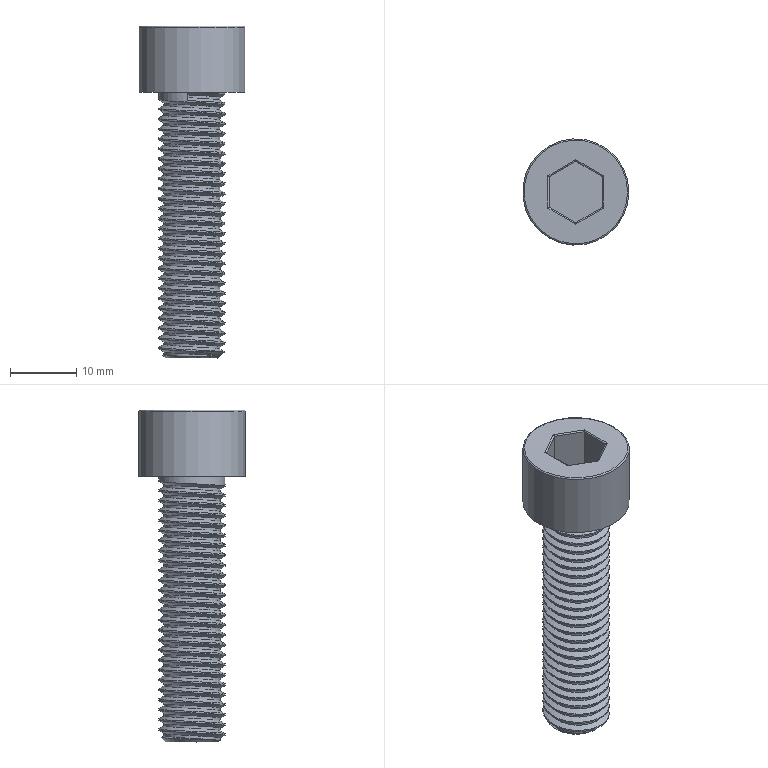Part | STEP file | Tube feed_id1730_x_t | 1 solid | 26 faces | box 16 x 16 x 50 mm | volume 4036 mm3 | plane 11 | cylinder 9 | spline 3 | cone 2 | torus 1 | commonest cylinder face diameters 0.4 x6 8.5 x1 10 x1 16 x1